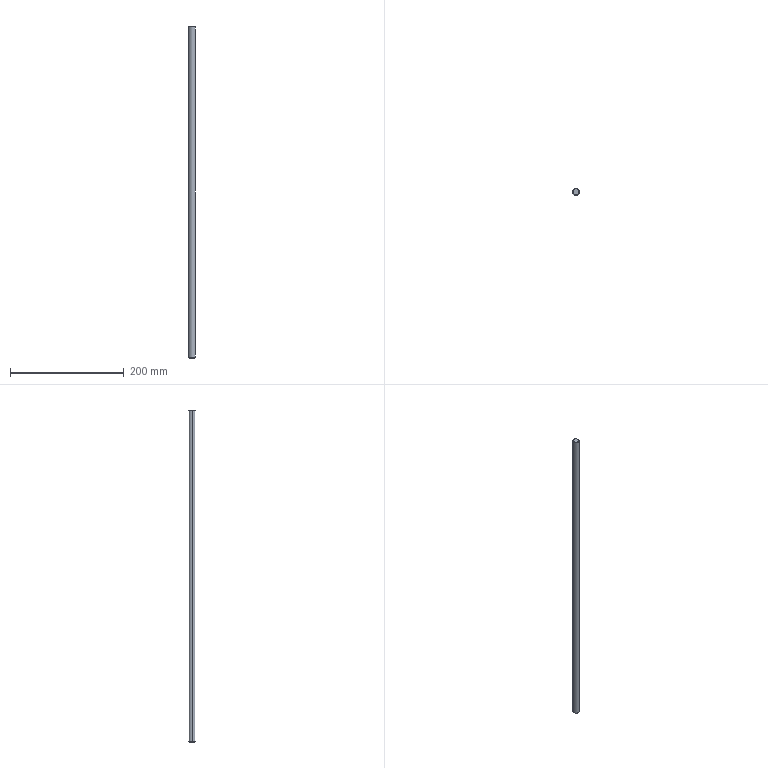Part | SolidWorks | features BaseBody 1 | 1 solid | 20 faces | box 12 x 12 x 584 mm | volume 65832 mm3 | cylinder 8 | plane 8 | cone 4 | commonest cylinder face diameters 3 x6 12 x2
STEP:
#1=CARTESIAN_POINT('',(4.2,0.,-284.));
#2=VERTEX_POINT('',#1);
#3=CARTESIAN_POINT('',(4.2,1.5,-282.5));
#4=VERTEX_POINT('',#3);
#5=CARTESIAN_POINT('',(4.2,0.,-282.5));
#6=DIRECTION('',(1.,0.,0.));
#7=DIRECTION('',(0.,0.,-1.));
#8=AXIS2_PLACEMENT_3D('',#5,#6,#7);
#9=CIRCLE('',#8,1.5);
#10=EDGE_CURVE('',#2,#4,#9,.T.);
#11=ORIENTED_EDGE('',*,*,#10,.F.);
#12=CARTESIAN_POINT('',(6.,0.,-284.));
#13=VERTEX_POINT('',#12);
#14=CARTESIAN_POINT('',(4.2,0.,-284.));
#15=DIRECTION('',(1.,0.,0.));
#16=VECTOR('',#15,1000.);
#17=LINE('',#14,#16);
#18=EDGE_CURVE('',#2,#13,#17,.T.);
#19=ORIENTED_EDGE('',*,*,#18,.T.);
#20=CARTESIAN_POINT('',(5.809,1.5,-282.5));
#21=VERTEX_POINT('',#20);
#22=CARTESIAN_POINT('',(5.809,1.5,-282.5));
#23=CARTESIAN_POINT('',(5.809,1.5,-282.6));
#24=CARTESIAN_POINT('',(5.812,1.49,-282.697));
#25=CARTESIAN_POINT('',(5.822,1.452,-282.89));
#26=CARTESIAN_POINT('',(5.829,1.423,-282.985));
#27=CARTESIAN_POINT('',(5.847,1.347,-283.167));
#28=CARTESIAN_POINT('',(5.857,1.301,-283.253));
#29=CARTESIAN_POINT('',(5.881,1.192,-283.415));
#30=CARTESIAN_POINT('',(5.893,1.129,-283.492));
#31=CARTESIAN_POINT('',(5.93,0.9223,-283.699));
#32=CARTESIAN_POINT('',(5.955,0.7555,-283.81));
#33=CARTESIAN_POINT('',(5.99,0.3946,-283.96));
#34=CARTESIAN_POINT('',(6.,0.1966,-284.));
#35=CARTESIAN_POINT('',(6.,0.,-284.));
#36=B_SPLINE_CURVE_WITH_KNOTS('',3,(#22,#23,#24,#25,#26,#27,#28,#29,#30,#31,#32,#33,#34,#35),.UNSPECIFIED.,.F.,.F.,(4,2,2,2,2,2,4),(0.,0.0002944,0.0005887,0.0008831,0.001177,0.001766,0.002355),.UNSPECIFIED.);
#37=EDGE_CURVE('',#21,#13,#36,.T.);
#38=ORIENTED_EDGE('',*,*,#37,.F.);
#39=CARTESIAN_POINT('',(4.2,1.5,-282.5));
#40=DIRECTION('',(1.,0.,0.));
#41=VECTOR('',#40,1000.);
#42=LINE('',#39,#41);
#43=EDGE_CURVE('',#4,#21,#42,.T.);
#44=ORIENTED_EDGE('',*,*,#43,.F.);
#45=EDGE_LOOP('',(#11,#19,#38,#44));
#46=FACE_OUTER_BOUND('',#45,.T.);
#47=CARTESIAN_POINT('',(4.2,0.,-282.5));
#48=DIRECTION('',(1.,0.,0.));
#49=DIRECTION('',(0.,0.,-1.));
#50=AXIS2_PLACEMENT_3D('',#47,#48,#49);
#51=CYLINDRICAL_SURFACE('',#50,1.5);
#52=ADVANCED_FACE('',(#46),#51,.F.);
#53=CARTESIAN_POINT('',(4.2,0.,266.));
#54=VERTEX_POINT('',#53);
#55=CARTESIAN_POINT('',(4.2,1.5,267.5));
#56=VERTEX_POINT('',#55);
#57=CARTESIAN_POINT('',(4.2,0.,267.5));
#58=DIRECTION('',(1.,0.,0.));
#59=DIRECTION('',(0.,0.,1.));
#60=AXIS2_PLACEMENT_3D('',#57,#58,#59);
#61=CIRCLE('',#60,1.5);
#62=EDGE_CURVE('',#54,#56,#61,.T.);
#63=ORIENTED_EDGE('',*,*,#62,.F.);
#64=CARTESIAN_POINT('',(6.,0.,266.));
#65=VERTEX_POINT('',#64);
#66=CARTESIAN_POINT('',(4.2,0.,266.));
#67=DIRECTION('',(1.,0.,0.));
#68=VECTOR('',#67,1000.);
#69=LINE('',#66,#68);
#70=EDGE_CURVE('',#54,#65,#69,.T.);
#71=ORIENTED_EDGE('',*,*,#70,.T.);
#72=CARTESIAN_POINT('',(5.809,1.5,267.5));
#73=VERTEX_POINT('',#72);
#74=CARTESIAN_POINT('',(5.809,1.5,267.5));
#75=CARTESIAN_POINT('',(5.809,1.5,267.4));
#76=CARTESIAN_POINT('',(5.812,1.49,267.303));
#77=CARTESIAN_POINT('',(5.822,1.452,267.11));
#78=CARTESIAN_POINT('',(5.829,1.423,267.015));
#79=CARTESIAN_POINT('',(5.847,1.347,266.833));
#80=CARTESIAN_POINT('',(5.857,1.301,266.747));
#81=CARTESIAN_POINT('',(5.881,1.192,266.585));
#82=CARTESIAN_POINT('',(5.893,1.129,266.508));
#83=CARTESIAN_POINT('',(5.93,0.9223,266.301));
#84=CARTESIAN_POINT('',(5.955,0.7555,266.19));
#85=CARTESIAN_POINT('',(5.99,0.3946,266.04));
#86=CARTESIAN_POINT('',(6.,0.1966,266.));
#87=CARTESIAN_POINT('',(6.,0.,266.));
#88=B_SPLINE_CURVE_WITH_KNOTS('',3,(#74,#75,#76,#77,#78,#79,#80,#81,#82,#83,#84,#85,#86,#87),.UNSPECIFIED.,.F.,.F.,(4,2,2,2,2,2,4),(0.,0.0002944,0.0005887,0.0008831,0.001177,0.001766,0.002355),.UNSPECIFIED.);
#89=EDGE_CURVE('',#73,#65,#88,.T.);
#90=ORIENTED_EDGE('',*,*,#89,.F.);
#91=CARTESIAN_POINT('',(4.2,1.5,267.5));
#92=DIRECTION('',(1.,0.,0.));
#93=VECTOR('',#92,1000.);
#94=LINE('',#91,#93);
#95=EDGE_CURVE('',#56,#73,#94,.T.);
#96=ORIENTED_EDGE('',*,*,#95,.F.);
#97=EDGE_LOOP('',(#63,#71,#90,#96));
#98=FACE_OUTER_BOUND('',#97,.T.);
#99=CARTESIAN_POINT('',(4.2,0.,267.5));
#100=DIRECTION('',(1.,0.,0.));
#101=DIRECTION('',(0.,0.,-1.));
#102=AXIS2_PLACEMENT_3D('',#99,#100,#101);
#103=CYLINDRICAL_SURFACE('',#102,1.5);
#104=ADVANCED_FACE('',(#98),#103,.F.);
#105=CARTESIAN_POINT('',(-5.,0.,-292.));
#106=VERTEX_POINT('',#105);
#107=CARTESIAN_POINT('',(5.,0.,-292.));
#108=VERTEX_POINT('',#107);
#109=CARTESIAN_POINT('',(0.,0.,-292.));
#110=DIRECTION('',(0.,0.,-1.));
#111=DIRECTION('',(1.,0.,0.));
#112=AXIS2_PLACEMENT_3D('',#109,#110,#111);
#113=CIRCLE('',#112,5.);
#114=EDGE_CURVE('',#106,#108,#113,.T.);
#115=ORIENTED_EDGE('',*,*,#114,.F.);
#116=CARTESIAN_POINT('',(-6.,0.,-291.));
#117=VERTEX_POINT('',#116);
#118=CARTESIAN_POINT('',(-6.,0.,-291.));
#119=DIRECTION('',(-0.7071,0.,0.7071));
#120=VECTOR('',#119,1000.);
#121=LINE('',#118,#120);
#122=EDGE_CURVE('',#106,#117,#121,.T.);
#123=ORIENTED_EDGE('',*,*,#122,.T.);
#124=CARTESIAN_POINT('',(6.,0.,-291.));
#125=VERTEX_POINT('',#124);
#126=CARTESIAN_POINT('',(0.,0.,-291.));
#127=DIRECTION('',(0.,0.,1.));
#128=DIRECTION('',(1.,0.,0.));
#129=AXIS2_PLACEMENT_3D('',#126,#127,#128);
#130=CIRCLE('',#129,6.);
#131=EDGE_CURVE('',#125,#117,#130,.T.);
#132=ORIENTED_EDGE('',*,*,#131,.F.);
#133=CARTESIAN_POINT('',(6.,0.,-291.));
#134=DIRECTION('',(0.7071,0.,0.7071));
#135=VECTOR('',#134,1000.);
#136=LINE('',#133,#135);
#137=EDGE_CURVE('',#108,#125,#136,.T.);
#138=ORIENTED_EDGE('',*,*,#137,.F.);
#139=EDGE_LOOP('',(#115,#123,#132,#138));
#140=FACE_OUTER_BOUND('',#139,.T.);
#141=CARTESIAN_POINT('',(0.,0.,-291.));
#142=DIRECTION('',(0.,0.,1.));
#143=DIRECTION('',(1.,0.,0.));
#144=AXIS2_PLACEMENT_3D('',#141,#142,#143);
#145=CONICAL_SURFACE('',#144,6.,0.7854);
#146=ADVANCED_FACE('',(#140),#145,.T.);
#147=CARTESIAN_POINT('',(5.,0.,292.));
#148=VERTEX_POINT('',#147);
#149=CARTESIAN_POINT('',(-5.,0.,292.));
#150=VERTEX_POINT('',#149);
#151=CARTESIAN_POINT('',(0.,0.,292.));
#152=DIRECTION('',(0.,0.,1.));
#153=DIRECTION('',(1.,0.,0.));
#154=AXIS2_PLACEMENT_3D('',#151,#152,#153);
#155=CIRCLE('',#154,5.);
#156=EDGE_CURVE('',#148,#150,#155,.T.);
#157=ORIENTED_EDGE('',*,*,#156,.F.);
#158=CARTESIAN_POINT('',(6.,0.,291.));
#159=VERTEX_POINT('',#158);
#160=CARTESIAN_POINT('',(5.,0.,292.));
#161=DIRECTION('',(0.7071,0.,-0.7071));
#162=VECTOR('',#161,1000.);
#163=LINE('',#160,#162);
#164=EDGE_CURVE('',#148,#159,#163,.T.);
#165=ORIENTED_EDGE('',*,*,#164,.T.);
#166=CARTESIAN_POINT('',(-6.,0.,291.));
#167=VERTEX_POINT('',#166);
#168=CARTESIAN_POINT('',(0.,0.,291.));
#169=DIRECTION('',(0.,0.,-1.));
#170=DIRECTION('',(1.,0.,0.));
#171=AXIS2_PLACEMENT_3D('',#168,#169,#170);
#172=CIRCLE('',#171,6.);
#173=EDGE_CURVE('',#167,#159,#172,.T.);
#174=ORIENTED_EDGE('',*,*,#173,.F.);
#175=CARTESIAN_POINT('',(-5.,0.,292.));
#176=DIRECTION('',(-0.7071,0.,-0.7071));
#177=VECTOR('',#176,1000.);
#178=LINE('',#175,#177);
#179=EDGE_CURVE('',#150,#167,#178,.T.);
#180=ORIENTED_EDGE('',*,*,#179,.F.);
#181=EDGE_LOOP('',(#157,#165,#174,#180));
#182=FACE_OUTER_BOUND('',#181,.T.);
#183=CARTESIAN_POINT('',(0.,0.,292.));
#184=DIRECTION('',(0.,0.,-1.));
#185=DIRECTION('',(-1.,0.,0.));
#186=AXIS2_PLACEMENT_3D('',#183,#184,#185);
#187=CONICAL_SURFACE('',#186,5.,0.7854);
#188=ADVANCED_FACE('',(#182),#187,.T.);
#189=ORIENTED_EDGE('',*,*,#173,.T.);
#190=CARTESIAN_POINT('',(6.,0.,284.));
#191=VERTEX_POINT('',#190);
#192=CARTESIAN_POINT('',(6.,0.,292.));
#193=DIRECTION('',(0.,0.,-1.));
#194=VECTOR('',#193,1000.);
#195=LINE('',#192,#194);
#196=EDGE_CURVE('',#159,#191,#195,.T.);
#197=ORIENTED_EDGE('',*,*,#196,.T.);
#198=CARTESIAN_POINT('',(5.809,1.5,282.5));
#199=VERTEX_POINT('',#198);
#200=CARTESIAN_POINT('',(6.,0.,284.));
#201=CARTESIAN_POINT('',(6.,0.1962,284.));
#202=CARTESIAN_POINT('',(5.99,0.3944,283.96));
#203=CARTESIAN_POINT('',(5.964,0.6654,283.848));
#204=CARTESIAN_POINT('',(5.953,0.7532,283.801));
#205=CARTESIAN_POINT('',(5.93,0.916,283.692));
#206=CARTESIAN_POINT('',(5.918,0.9912,283.63));
#207=CARTESIAN_POINT('',(5.893,1.13,283.492));
#208=CARTESIAN_POINT('',(5.881,1.193,283.415));
#209=CARTESIAN_POINT('',(5.858,1.301,283.253));
#210=CARTESIAN_POINT('',(5.847,1.347,283.167));
#211=CARTESIAN_POINT('',(5.82,1.461,282.893));
#212=CARTESIAN_POINT('',(5.809,1.5,282.698));
#213=CARTESIAN_POINT('',(5.809,1.5,282.5));
#214=B_SPLINE_CURVE_WITH_KNOTS('',3,(#200,#201,#202,#203,#204,#205,#206,#207,#208,#209,#210,#211,#212,#213),.UNSPECIFIED.,.F.,.F.,(4,2,2,2,2,2,4),(0.004708,0.005297,0.005591,0.005885,0.00618,0.006474,0.007062),.UNSPECIFIED.);
#215=EDGE_CURVE('',#191,#199,#214,.T.);
#216=ORIENTED_EDGE('',*,*,#215,.T.);
#217=CARTESIAN_POINT('',(5.809,1.5,292.));
#218=DIRECTION('',(0.,0.,-1.));
#219=VECTOR('',#218,1000.);
#220=LINE('',#217,#219);
#221=EDGE_CURVE('',#199,#73,#220,.T.);
#222=ORIENTED_EDGE('',*,*,#221,.T.);
#223=ORIENTED_EDGE('',*,*,#89,.T.);
#224=CARTESIAN_POINT('',(6.,0.,-266.));
#225=VERTEX_POINT('',#224);
#226=CARTESIAN_POINT('',(6.,0.,292.));
#227=DIRECTION('',(0.,0.,-1.));
#228=VECTOR('',#227,1000.);
#229=LINE('',#226,#228);
#230=EDGE_CURVE('',#65,#225,#229,.T.);
#231=ORIENTED_EDGE('',*,*,#230,.T.);
#232=CARTESIAN_POINT('',(5.809,1.5,-267.5));
#233=VERTEX_POINT('',#232);
#234=CARTESIAN_POINT('',(6.,0.,-266.));
#235=CARTESIAN_POINT('',(6.,0.1962,-266.));
#236=CARTESIAN_POINT('',(5.99,0.3944,-266.04));
#237=CARTESIAN_POINT('',(5.964,0.6654,-266.152));
#238=CARTESIAN_POINT('',(5.953,0.7532,-266.199));
#239=CARTESIAN_POINT('',(5.93,0.916,-266.308));
#240=CARTESIAN_POINT('',(5.918,0.9912,-266.37));
#241=CARTESIAN_POINT('',(5.893,1.13,-266.508));
#242=CARTESIAN_POINT('',(5.881,1.193,-266.585));
#243=CARTESIAN_POINT('',(5.858,1.301,-266.747));
#244=CARTESIAN_POINT('',(5.847,1.347,-266.833));
#245=CARTESIAN_POINT('',(5.82,1.461,-267.107));
#246=CARTESIAN_POINT('',(5.809,1.5,-267.302));
#247=CARTESIAN_POINT('',(5.809,1.5,-267.5));
#248=B_SPLINE_CURVE_WITH_KNOTS('',3,(#234,#235,#236,#237,#238,#239,#240,#241,#242,#243,#244,#245,#246,#247),.UNSPECIFIED.,.F.,.F.,(4,2,2,2,2,2,4),(0.004708,0.005297,0.005591,0.005885,0.00618,0.006474,0.007062),.UNSPECIFIED.);
#249=EDGE_CURVE('',#225,#233,#248,.T.);
#250=ORIENTED_EDGE('',*,*,#249,.T.);
#251=CARTESIAN_POINT('',(5.809,1.5,292.));
#252=DIRECTION('',(0.,0.,-1.));
#253=VECTOR('',#252,1000.);
#254=LINE('',#251,#253);
#255=EDGE_CURVE('',#233,#21,#254,.T.);
#256=ORIENTED_EDGE('',*,*,#255,.T.);
#257=ORIENTED_EDGE('',*,*,#37,.T.);
#258=CARTESIAN_POINT('',(6.,0.,292.));
#259=DIRECTION('',(0.,0.,-1.));
#260=VECTOR('',#259,1000.);
#261=LINE('',#258,#260);
#262=EDGE_CURVE('',#13,#125,#261,.T.);
#263=ORIENTED_EDGE('',*,*,#262,.T.);
#264=ORIENTED_EDGE('',*,*,#131,.T.);
#265=CARTESIAN_POINT('',(-6.,0.,292.));
#266=DIRECTION('',(0.,0.,-1.));
#267=VECTOR('',#266,1000.);
#268=LINE('',#265,#267);
#269=EDGE_CURVE('',#167,#117,#268,.T.);
#270=ORIENTED_EDGE('',*,*,#269,.F.);
#271=EDGE_LOOP('',(#189,#197,#216,#222,#223,#231,#250,#256,#257,#263,#264,#270));
#272=FACE_OUTER_BOUND('',#271,.T.);
#273=CARTESIAN_POINT('',(0.,0.,292.));
#274=DIRECTION('',(0.,0.,-1.));
#275=DIRECTION('',(-1.,0.,0.));
#276=AXIS2_PLACEMENT_3D('',#273,#274,#275);
#277=CYLINDRICAL_SURFACE('',#276,6.);
#278=ADVANCED_FACE('',(#272),#277,.T.);
#279=ORIENTED_EDGE('',*,*,#196,.F.);
#280=CARTESIAN_POINT('',(0.,0.,291.));
#281=DIRECTION('',(0.,0.,-1.));
#282=DIRECTION('',(1.,0.,0.));
#283=AXIS2_PLACEMENT_3D('',#280,#281,#282);
#284=CIRCLE('',#283,6.);
#285=EDGE_CURVE('',#159,#167,#284,.T.);
#286=ORIENTED_EDGE('',*,*,#285,.T.);
#287=ORIENTED_EDGE('',*,*,#269,.T.);
#288=CARTESIAN_POINT('',(0.,0.,-291.));
#289=DIRECTION('',(0.,0.,1.));
#290=DIRECTION('',(1.,0.,0.));
#291=AXIS2_PLACEMENT_3D('',#288,#289,#290);
#292=CIRCLE('',#291,6.);
#293=EDGE_CURVE('',#117,#125,#292,.T.);
#294=ORIENTED_EDGE('',*,*,#293,.T.);
#295=ORIENTED_EDGE('',*,*,#262,.F.);
#296=CARTESIAN_POINT('',(5.809,-1.5,-282.5));
#297=VERTEX_POINT('',#296);
#298=CARTESIAN_POINT('',(6.,0.,-284.));
#299=CARTESIAN_POINT('',(6.,-0.0982,-284.));
#300=CARTESIAN_POINT('',(5.998,-0.198,-283.99));
#301=CARTESIAN_POINT('',(5.988,-0.3905,-283.952));
#302=CARTESIAN_POINT('',(5.981,-0.4841,-283.923));
#303=CARTESIAN_POINT('',(5.955,-0.7571,-283.81));
#304=CARTESIAN_POINT('',(5.93,-0.9218,-283.699));
#305=CARTESIAN_POINT('',(5.893,-1.13,-283.491));
#306=CARTESIAN_POINT('',(5.881,-1.192,-283.416));
#307=CARTESIAN_POINT('',(5.858,-1.3,-283.254));
#308=CARTESIAN_POINT('',(5.847,-1.347,-283.166));
#309=CARTESIAN_POINT('',(5.82,-1.46,-282.895));
#310=CARTESIAN_POINT('',(5.809,-1.5,-282.699));
#311=CARTESIAN_POINT('',(5.809,-1.5,-282.5));
#312=B_SPLINE_CURVE_WITH_KNOTS('',3,(#298,#299,#300,#301,#302,#303,#304,#305,#306,#307,#308,#309,#310,#311),.UNSPECIFIED.,.F.,.F.,(4,2,2,2,2,2,4),(0.002355,0.002649,0.002943,0.003531,0.003825,0.004119,0.004707),.UNSPECIFIED.);
#313=EDGE_CURVE('',#13,#297,#312,.T.);
#314=ORIENTED_EDGE('',*,*,#313,.T.);
#315=CARTESIAN_POINT('',(5.809,-1.5,-267.5));
#316=VERTEX_POINT('',#315);
#317=CARTESIAN_POINT('',(5.809,-1.5,292.));
#318=DIRECTION('',(0.,0.,1.));
#319=VECTOR('',#318,1000.);
#320=LINE('',#317,#319);
#321=EDGE_CURVE('',#297,#316,#320,.T.);
#322=ORIENTED_EDGE('',*,*,#321,.T.);
#323=CARTESIAN_POINT('',(5.809,-1.5,-267.5));
#324=CARTESIAN_POINT('',(5.809,-1.5,-267.402));
#325=CARTESIAN_POINT('',(5.812,-1.49,-267.302));
#326=CARTESIAN_POINT('',(5.822,-1.452,-267.109));
#327=CARTESIAN_POINT('',(5.829,-1.423,-267.016));
#328=CARTESIAN_POINT('',(5.856,-1.31,-266.743));
#329=CARTESIAN_POINT('',(5.881,-1.199,-266.578));
#330=CARTESIAN_POINT('',(5.918,-0.9907,-266.369));
#331=CARTESIAN_POINT('',(5.93,-0.9154,-266.308));
#332=CARTESIAN_POINT('',(5.953,-0.7533,-266.199));
#333=CARTESIAN_POINT('',(5.964,-0.6654,-266.152));
#334=CARTESIAN_POINT('',(5.981,-0.4843,-266.077));
#335=CARTESIAN_POINT('',(5.988,-0.3908,-266.048));
#336=CARTESIAN_POINT('',(5.998,-0.1977,-266.01));
#337=CARTESIAN_POINT('',(6.,-0.0981,-266.));
#338=CARTESIAN_POINT('',(6.,0.,-266.));
#339=B_SPLINE_CURVE_WITH_KNOTS('',3,(#323,#324,#325,#326,#327,#328,#329,#330,#331,#332,#333,#334,#335,#336,#337,#338),.UNSPECIFIED.,.F.,.F.,(4,2,2,2,2,2,2,4),(0.002355,0.002649,0.002943,0.003532,0.003826,0.00412,0.004414,0.004708),.UNSPECIFIED.);
#340=EDGE_CURVE('',#316,#225,#339,.T.);
#341=ORIENTED_EDGE('',*,*,#340,.T.);
#342=ORIENTED_EDGE('',*,*,#230,.F.);
#343=CARTESIAN_POINT('',(5.809,-1.5,267.5));
#344=VERTEX_POINT('',#343);
#345=CARTESIAN_POINT('',(6.,0.,266.));
#346=CARTESIAN_POINT('',(6.,-0.0982,266.));
#347=CARTESIAN_POINT('',(5.998,-0.198,266.01));
#348=CARTESIAN_POINT('',(5.988,-0.3905,266.048));
#349=CARTESIAN_POINT('',(5.981,-0.4841,266.077));
#350=CARTESIAN_POINT('',(5.955,-0.7571,266.19));
#351=CARTESIAN_POINT('',(5.93,-0.9218,266.301));
#352=CARTESIAN_POINT('',(5.893,-1.13,266.509));
#353=CARTESIAN_POINT('',(5.881,-1.192,266.584));
#354=CARTESIAN_POINT('',(5.858,-1.3,266.746));
#355=CARTESIAN_POINT('',(5.847,-1.347,266.834));
#356=CARTESIAN_POINT('',(5.82,-1.46,267.105));
#357=CARTESIAN_POINT('',(5.809,-1.5,267.301));
#358=CARTESIAN_POINT('',(5.809,-1.5,267.5));
#359=B_SPLINE_CURVE_WITH_KNOTS('',3,(#345,#346,#347,#348,#349,#350,#351,#352,#353,#354,#355,#356,#357,#358),.UNSPECIFIED.,.F.,.F.,(4,2,2,2,2,2,4),(0.002355,0.002649,0.002943,0.003531,0.003825,0.004119,0.004707),.UNSPECIFIED.);
#360=EDGE_CURVE('',#65,#344,#359,.T.);
#361=ORIENTED_EDGE('',*,*,#360,.T.);
#362=CARTESIAN_POINT('',(5.809,-1.5,282.5));
#363=VERTEX_POINT('',#362);
#364=CARTESIAN_POINT('',(5.809,-1.5,292.));
#365=DIRECTION('',(0.,0.,1.));
#366=VECTOR('',#365,1000.);
#367=LINE('',#364,#366);
#368=EDGE_CURVE('',#344,#363,#367,.T.);
#369=ORIENTED_EDGE('',*,*,#368,.T.);
#370=CARTESIAN_POINT('',(5.809,-1.5,282.5));
#371=CARTESIAN_POINT('',(5.809,-1.5,282.598));
#372=CARTESIAN_POINT('',(5.812,-1.49,282.698));
#373=CARTESIAN_POINT('',(5.822,-1.452,282.891));
#374=CARTESIAN_POINT('',(5.829,-1.423,282.984));
#375=CARTESIAN_POINT('',(5.856,-1.31,283.257));
#376=CARTESIAN_POINT('',(5.881,-1.199,283.422));
#377=CARTESIAN_POINT('',(5.918,-0.9907,283.631));
#378=CARTESIAN_POINT('',(5.93,-0.9154,283.692));
#379=CARTESIAN_POINT('',(5.953,-0.7533,283.801));
#380=CARTESIAN_POINT('',(5.964,-0.6654,283.848));
#381=CARTESIAN_POINT('',(5.981,-0.4843,283.923));
#382=CARTESIAN_POINT('',(5.988,-0.3908,283.952));
#383=CARTESIAN_POINT('',(5.998,-0.1977,283.99));
#384=CARTESIAN_POINT('',(6.,-0.0981,284.));
#385=CARTESIAN_POINT('',(6.,0.,284.));
#386=B_SPLINE_CURVE_WITH_KNOTS('',3,(#370,#371,#372,#373,#374,#375,#376,#377,#378,#379,#380,#381,#382,#383,#384,#385),.UNSPECIFIED.,.F.,.F.,(4,2,2,2,2,2,2,4),(0.002355,0.002649,0.002943,0.003532,0.003826,0.00412,0.004414,0.004708),.UNSPECIFIED.);
#387=EDGE_CURVE('',#363,#191,#386,.T.);
#388=ORIENTED_EDGE('',*,*,#387,.T.);
#389=EDGE_LOOP('',(#279,#286,#287,#294,#295,#314,#322,#341,#342,#361,#369,#388));
#390=FACE_OUTER_BOUND('',#389,.T.);
#391=CARTESIAN_POINT('',(0.,0.,292.));
#392=DIRECTION('',(0.,0.,-1.));
#393=DIRECTION('',(-1.,0.,0.));
#394=AXIS2_PLACEMENT_3D('',#391,#392,#393);
#395=CYLINDRICAL_SURFACE('',#394,6.);
#396=ADVANCED_FACE('',(#390),#395,.T.);
#397=CARTESIAN_POINT('',(0.,0.,292.));
#398=DIRECTION('',(0.,0.,1.));
#399=DIRECTION('',(1.,0.,0.));
#400=AXIS2_PLACEMENT_3D('',#397,#398,#399);
#401=CIRCLE('',#400,5.);
#402=EDGE_CURVE('',#150,#148,#401,.T.);
#403=ORIENTED_EDGE('',*,*,#402,.T.);
#404=ORIENTED_EDGE('',*,*,#156,.T.);
#405=EDGE_LOOP('',(#403,#404));
#406=FACE_OUTER_BOUND('',#405,.T.);
#407=CARTESIAN_POINT('',(0.,0.,292.));
#408=DIRECTION('',(0.,0.,1.));
#409=DIRECTION('',(1.,0.,0.));
#410=AXIS2_PLACEMENT_3D('',#407,#408,#409);
#411=PLANE('',#410);
#412=ADVANCED_FACE('',(#406),#411,.T.);
#413=CARTESIAN_POINT('',(0.,0.,-292.));
#414=DIRECTION('',(0.,0.,-1.));
#415=DIRECTION('',(1.,0.,0.));
#416=AXIS2_PLACEMENT_3D('',#413,#414,#415);
#417=CIRCLE('',#416,5.);
#418=EDGE_CURVE('',#108,#106,#417,.T.);
#419=ORIENTED_EDGE('',*,*,#418,.T.);
#420=ORIENTED_EDGE('',*,*,#114,.T.);
#421=EDGE_LOOP('',(#419,#420));
#422=FACE_OUTER_BOUND('',#421,.T.);
#423=CARTESIAN_POINT('',(0.,0.,-292.));
#424=DIRECTION('',(0.,0.,1.));
#425=DIRECTION('',(1.,0.,0.));
#426=AXIS2_PLACEMENT_3D('',#423,#424,#425);
#427=PLANE('',#426);
#428=ADVANCED_FACE('',(#422),#427,.F.);
#429=ORIENTED_EDGE('',*,*,#164,.F.);
#430=ORIENTED_EDGE('',*,*,#402,.F.);
#431=ORIENTED_EDGE('',*,*,#179,.T.);
#432=ORIENTED_EDGE('',*,*,#285,.F.);
#433=EDGE_LOOP('',(#429,#430,#431,#432));
#434=FACE_OUTER_BOUND('',#433,.T.);
#435=CARTESIAN_POINT('',(0.,0.,292.));
#436=DIRECTION('',(0.,0.,-1.));
#437=DIRECTION('',(-1.,0.,0.));
#438=AXIS2_PLACEMENT_3D('',#435,#436,#437);
#439=CONICAL_SURFACE('',#438,5.,0.7854);
#440=ADVANCED_FACE('',(#434),#439,.T.);
#441=ORIENTED_EDGE('',*,*,#122,.F.);
#442=ORIENTED_EDGE('',*,*,#418,.F.);
#443=ORIENTED_EDGE('',*,*,#137,.T.);
#444=ORIENTED_EDGE('',*,*,#293,.F.);
#445=EDGE_LOOP('',(#441,#442,#443,#444));
#446=FACE_OUTER_BOUND('',#445,.T.);
#447=CARTESIAN_POINT('',(0.,0.,-291.));
#448=DIRECTION('',(0.,0.,1.));
#449=DIRECTION('',(1.,0.,0.));
#450=AXIS2_PLACEMENT_3D('',#447,#448,#449);
#451=CONICAL_SURFACE('',#450,6.,0.7854);
#452=ADVANCED_FACE('',(#446),#451,.T.);
#453=CARTESIAN_POINT('',(4.2,-1.5,282.5));
#454=VERTEX_POINT('',#453);
#455=CARTESIAN_POINT('',(4.2,-1.5,282.5));
#456=DIRECTION('',(1.,0.,0.));
#457=VECTOR('',#456,1000.);
#458=LINE('',#455,#457);
#459=EDGE_CURVE('',#454,#363,#458,.T.);
#460=ORIENTED_EDGE('',*,*,#459,.F.);
#461=CARTESIAN_POINT('',(4.2,1.5,282.5));
#462=VERTEX_POINT('',#461);
#463=CARTESIAN_POINT('',(4.2,0.,282.5));
#464=DIRECTION('',(1.,0.,0.));
#465=DIRECTION('',(0.,0.,1.));
#466=AXIS2_PLACEMENT_3D('',#463,#464,#465);
#467=CIRCLE('',#466,1.5);
#468=EDGE_CURVE('',#462,#454,#467,.T.);
#469=ORIENTED_EDGE('',*,*,#468,.F.);
#470=CARTESIAN_POINT('',(4.2,1.5,282.5));
#471=DIRECTION('',(1.,0.,0.));
#472=VECTOR('',#471,1000.);
#473=LINE('',#470,#472);
#474=EDGE_CURVE('',#462,#199,#473,.T.);
#475=ORIENTED_EDGE('',*,*,#474,.T.);
#476=ORIENTED_EDGE('',*,*,#215,.F.);
#477=ORIENTED_EDGE('',*,*,#387,.F.);
#478=EDGE_LOOP('',(#460,#469,#475,#476,#477));
#479=FACE_OUTER_BOUND('',#478,.T.);
#480=CARTESIAN_POINT('',(4.2,0.,282.5));
#481=DIRECTION('',(1.,0.,0.));
#482=DIRECTION('',(0.,0.,-1.));
#483=AXIS2_PLACEMENT_3D('',#480,#481,#482);
#484=CYLINDRICAL_SURFACE('',#483,1.5);
#485=ADVANCED_FACE('',(#479),#484,.F.);
#486=ORIENTED_EDGE('',*,*,#474,.F.);
#487=CARTESIAN_POINT('',(4.2,1.5,282.5));
#488=DIRECTION('',(0.,0.,1.));
#489=VECTOR('',#488,1000.);
#490=LINE('',#487,#489);
#491=EDGE_CURVE('',#56,#462,#490,.T.);
#492=ORIENTED_EDGE('',*,*,#491,.F.);
#493=ORIENTED_EDGE('',*,*,#95,.T.);
#494=ORIENTED_EDGE('',*,*,#221,.F.);
#495=EDGE_LOOP('',(#486,#492,#493,#494));
#496=FACE_OUTER_BOUND('',#495,.T.);
#497=CARTESIAN_POINT('',(4.2,1.5,282.5));
#498=DIRECTION('',(0.,1.,0.));
#499=DIRECTION('',(0.,0.,1.));
#500=AXIS2_PLACEMENT_3D('',#497,#498,#499);
#501=PLANE('',#500);
#502=ADVANCED_FACE('',(#496),#501,.F.);
#503=ORIENTED_EDGE('',*,*,#70,.F.);
#504=CARTESIAN_POINT('',(4.2,-1.5,267.5));
#505=VERTEX_POINT('',#504);
#506=CARTESIAN_POINT('',(4.2,0.,267.5));
#507=DIRECTION('',(1.,0.,0.));
#508=DIRECTION('',(0.,0.,1.));
#509=AXIS2_PLACEMENT_3D('',#506,#507,#508);
#510=CIRCLE('',#509,1.5);
#511=EDGE_CURVE('',#505,#54,#510,.T.);
#512=ORIENTED_EDGE('',*,*,#511,.F.);
#513=CARTESIAN_POINT('',(4.2,-1.5,267.5));
#514=DIRECTION('',(1.,0.,0.));
#515=VECTOR('',#514,1000.);
#516=LINE('',#513,#515);
#517=EDGE_CURVE('',#505,#344,#516,.T.);
#518=ORIENTED_EDGE('',*,*,#517,.T.);
#519=ORIENTED_EDGE('',*,*,#360,.F.);
#520=EDGE_LOOP('',(#503,#512,#518,#519));
#521=FACE_OUTER_BOUND('',#520,.T.);
#522=CARTESIAN_POINT('',(4.2,0.,267.5));
#523=DIRECTION('',(1.,0.,0.));
#524=DIRECTION('',(0.,0.,-1.));
#525=AXIS2_PLACEMENT_3D('',#522,#523,#524);
#526=CYLINDRICAL_SURFACE('',#525,1.5);
#527=ADVANCED_FACE('',(#521),#526,.F.);
#528=ORIENTED_EDGE('',*,*,#517,.F.);
#529=CARTESIAN_POINT('',(4.2,-1.5,282.5));
#530=DIRECTION('',(0.,0.,-1.));
#531=VECTOR('',#530,1000.);
#532=LINE('',#529,#531);
#533=EDGE_CURVE('',#454,#505,#532,.T.);
#534=ORIENTED_EDGE('',*,*,#533,.F.);
#535=ORIENTED_EDGE('',*,*,#459,.T.);
#536=ORIENTED_EDGE('',*,*,#368,.F.);
#537=EDGE_LOOP('',(#528,#534,#535,#536));
#538=FACE_OUTER_BOUND('',#537,.T.);
#539=CARTESIAN_POINT('',(4.2,-1.5,282.5));
#540=DIRECTION('',(0.,-1.,0.));
#541=DIRECTION('',(0.,0.,-1.));
#542=AXIS2_PLACEMENT_3D('',#539,#540,#541);
#543=PLANE('',#542);
#544=ADVANCED_FACE('',(#538),#543,.F.);
#545=ORIENTED_EDGE('',*,*,#468,.T.);
#546=ORIENTED_EDGE('',*,*,#533,.T.);
#547=ORIENTED_EDGE('',*,*,#511,.T.);
#548=ORIENTED_EDGE('',*,*,#62,.T.);
#549=ORIENTED_EDGE('',*,*,#491,.T.);
#550=EDGE_LOOP('',(#545,#546,#547,#548,#549));
#551=FACE_OUTER_BOUND('',#550,.T.);
#552=CARTESIAN_POINT('',(4.2,0.,282.5));
#553=DIRECTION('',(-1.,0.,0.));
#554=DIRECTION('',(0.,0.,1.));
#555=AXIS2_PLACEMENT_3D('',#552,#553,#554);
#556=PLANE('',#555);
#557=ADVANCED_FACE('',(#551),#556,.F.);
#558=ORIENTED_EDGE('',*,*,#18,.F.);
#559=CARTESIAN_POINT('',(4.2,-1.5,-282.5));
#560=VERTEX_POINT('',#559);
#561=CARTESIAN_POINT('',(4.2,0.,-282.5));
#562=DIRECTION('',(1.,0.,0.));
#563=DIRECTION('',(0.,0.,-1.));
#564=AXIS2_PLACEMENT_3D('',#561,#562,#563);
#565=CIRCLE('',#564,1.5);
#566=EDGE_CURVE('',#560,#2,#565,.T.);
#567=ORIENTED_EDGE('',*,*,#566,.F.);
#568=CARTESIAN_POINT('',(4.2,-1.5,-282.5));
#569=DIRECTION('',(1.,0.,0.));
#570=VECTOR('',#569,1000.);
#571=LINE('',#568,#570);
#572=EDGE_CURVE('',#560,#297,#571,.T.);
#573=ORIENTED_EDGE('',*,*,#572,.T.);
#574=ORIENTED_EDGE('',*,*,#313,.F.);
#575=EDGE_LOOP('',(#558,#567,#573,#574));
#576=FACE_OUTER_BOUND('',#575,.T.);
#577=CARTESIAN_POINT('',(4.2,0.,-282.5));
#578=DIRECTION('',(1.,0.,0.));
#579=DIRECTION('',(0.,0.,-1.));
#580=AXIS2_PLACEMENT_3D('',#577,#578,#579);
#581=CYLINDRICAL_SURFACE('',#580,1.5);
#582=ADVANCED_FACE('',(#576),#581,.F.);
#583=ORIENTED_EDGE('',*,*,#572,.F.);
#584=CARTESIAN_POINT('',(4.2,-1.5,-267.5));
#585=VERTEX_POINT('',#584);
#586=CARTESIAN_POINT('',(4.2,-1.5,-282.5));
#587=DIRECTION('',(0.,0.,-1.));
#588=VECTOR('',#587,1000.);
#589=LINE('',#586,#588);
#590=EDGE_CURVE('',#585,#560,#589,.T.);
#591=ORIENTED_EDGE('',*,*,#590,.F.);
#592=CARTESIAN_POINT('',(4.2,-1.5,-267.5));
#593=DIRECTION('',(1.,0.,0.));
#594=VECTOR('',#593,1000.);
#595=LINE('',#592,#594);
#596=EDGE_CURVE('',#585,#316,#595,.T.);
#597=ORIENTED_EDGE('',*,*,#596,.T.);
#598=ORIENTED_EDGE('',*,*,#321,.F.);
#599=EDGE_LOOP('',(#583,#591,#597,#598));
#600=FACE_OUTER_BOUND('',#599,.T.);
#601=CARTESIAN_POINT('',(4.2,-1.5,-282.5));
#602=DIRECTION('',(0.,-1.,0.));
#603=DIRECTION('',(0.,0.,-1.));
#604=AXIS2_PLACEMENT_3D('',#601,#602,#603);
#605=PLANE('',#604);
#606=ADVANCED_FACE('',(#600),#605,.F.);
#607=ORIENTED_EDGE('',*,*,#596,.F.);
#608=CARTESIAN_POINT('',(4.2,1.5,-267.5));
#609=VERTEX_POINT('',#608);
#610=CARTESIAN_POINT('',(4.2,0.,-267.5));
#611=DIRECTION('',(1.,0.,0.));
#612=DIRECTION('',(0.,0.,-1.));
#613=AXIS2_PLACEMENT_3D('',#610,#611,#612);
#614=CIRCLE('',#613,1.5);
#615=EDGE_CURVE('',#609,#585,#614,.T.);
#616=ORIENTED_EDGE('',*,*,#615,.F.);
#617=CARTESIAN_POINT('',(4.2,1.5,-267.5));
#618=DIRECTION('',(1.,0.,0.));
#619=VECTOR('',#618,1000.);
#620=LINE('',#617,#619);
#621=EDGE_CURVE('',#609,#233,#620,.T.);
#622=ORIENTED_EDGE('',*,*,#621,.T.);
#623=ORIENTED_EDGE('',*,*,#249,.F.);
#624=ORIENTED_EDGE('',*,*,#340,.F.);
#625=EDGE_LOOP('',(#607,#616,#622,#623,#624));
#626=FACE_OUTER_BOUND('',#625,.T.);
#627=CARTESIAN_POINT('',(4.2,0.,-267.5));
#628=DIRECTION('',(1.,0.,0.));
#629=DIRECTION('',(0.,0.,-1.));
#630=AXIS2_PLACEMENT_3D('',#627,#628,#629);
#631=CYLINDRICAL_SURFACE('',#630,1.5);
#632=ADVANCED_FACE('',(#626),#631,.F.);
#633=ORIENTED_EDGE('',*,*,#621,.F.);
#634=CARTESIAN_POINT('',(4.2,1.5,-282.5));
#635=DIRECTION('',(0.,0.,1.));
#636=VECTOR('',#635,1000.);
#637=LINE('',#634,#636);
#638=EDGE_CURVE('',#4,#609,#637,.T.);
#639=ORIENTED_EDGE('',*,*,#638,.F.);
#640=ORIENTED_EDGE('',*,*,#43,.T.);
#641=ORIENTED_EDGE('',*,*,#255,.F.);
#642=EDGE_LOOP('',(#633,#639,#640,#641));
#643=FACE_OUTER_BOUND('',#642,.T.);
#644=CARTESIAN_POINT('',(4.2,1.5,-282.5));
#645=DIRECTION('',(0.,1.,0.));
#646=DIRECTION('',(0.,0.,1.));
#647=AXIS2_PLACEMENT_3D('',#644,#645,#646);
#648=PLANE('',#647);
#649=ADVANCED_FACE('',(#643),#648,.F.);
#650=ORIENTED_EDGE('',*,*,#566,.T.);
#651=ORIENTED_EDGE('',*,*,#10,.T.);
#652=ORIENTED_EDGE('',*,*,#638,.T.);
#653=ORIENTED_EDGE('',*,*,#615,.T.);
#654=ORIENTED_EDGE('',*,*,#590,.T.);
#655=EDGE_LOOP('',(#650,#651,#652,#653,#654));
#656=FACE_OUTER_BOUND('',#655,.T.);
#657=CARTESIAN_POINT('',(4.2,0.,-282.5));
#658=DIRECTION('',(1.,0.,0.));
#659=DIRECTION('',(0.,0.,-1.));
#660=AXIS2_PLACEMENT_3D('',#657,#658,#659);
#661=PLANE('',#660);
#662=ADVANCED_FACE('',(#656),#661,.T.);
#663=CLOSED_SHELL('',(#52,#104,#146,#188,#278,#396,#412,#428,#440,#452,#485,#502,#527,#544,#557,#582,#606,#632,#649,#662));
#664=MANIFOLD_SOLID_BREP('',#663);
#665=CARTESIAN_POINT('',(0.,0.,0.));
#666=DIRECTION('',(0.,0.,1.));
#667=DIRECTION('',(1.,0.,0.));
#668=AXIS2_PLACEMENT_3D('',#665,#666,#667);
#669=(LENGTH_UNIT()NAMED_UNIT(*)SI_UNIT(.MILLI.,.METRE.));
#670=UNCERTAINTY_MEASURE_WITH_UNIT(LENGTH_MEASURE(0.00001),#669,'','');
#671=(NAMED_UNIT(*)PLANE_ANGLE_UNIT()SI_UNIT($,.RADIAN.));
#672=(NAMED_UNIT(*)SI_UNIT($,.STERADIAN.)SOLID_ANGLE_UNIT());
#673=(GEOMETRIC_REPRESENTATION_CONTEXT(3)GLOBAL_UNCERTAINTY_ASSIGNED_CONTEXT((#670))GLOBAL_UNIT_ASSIGNED_CONTEXT((#669,#671,#672))REPRESENTATION_CONTEXT('',''));
#674=ADVANCED_BREP_SHAPE_REPRESENTATION('',(#664,#668),#673);